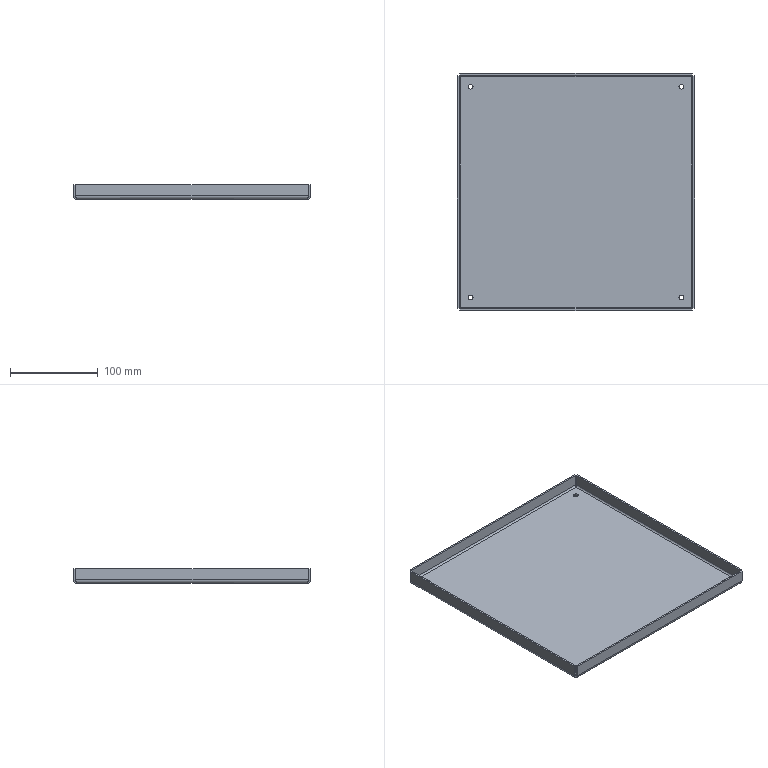Part | STEP file | Station two mount plate | 1 solid | 46 faces | box 270 x 270 x 17 mm | volume 174541 mm3 | plane 22 | cylinder 16 | spline 8 | commonest cylinder face diameters 5.5 x8 4 x4 8 x4